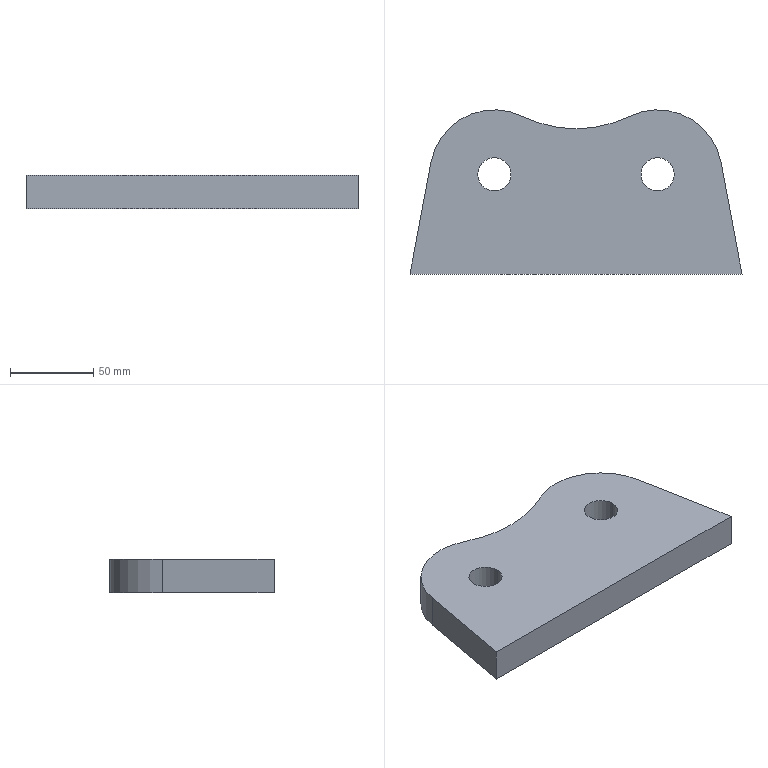Part | SolidWorks | features BaseBody 1 | 1 solid | 12 faces | box 200 x 98.946 x 20 mm | volume 325794 mm3 | cylinder 7 | plane 5 | commonest cylinder face diameters 20 x4 77.784 x2 145 x1
STEP:
#1=CARTESIAN_POINT('',(2641.622,1907.745,0.));
#2=VERTEX_POINT('',#1);
#3=CARTESIAN_POINT('',(2661.622,1907.745,0.));
#4=VERTEX_POINT('',#3);
#5=CARTESIAN_POINT('',(2651.622,1907.745,0.));
#6=DIRECTION('',(0.,0.,1.));
#7=DIRECTION('',(-1.,0.,0.));
#8=AXIS2_PLACEMENT_3D('',#5,#6,#7);
#9=CIRCLE('',#8,10.);
#10=EDGE_CURVE('',#2,#4,#9,.T.);
#11=ORIENTED_EDGE('',*,*,#10,.F.);
#12=CARTESIAN_POINT('',(2641.622,1907.745,20.));
#13=VERTEX_POINT('',#12);
#14=CARTESIAN_POINT('',(2641.622,1907.745,0.));
#15=DIRECTION('',(0.,0.,1.));
#16=VECTOR('',#15,1000.);
#17=LINE('',#14,#16);
#18=EDGE_CURVE('',#2,#13,#17,.T.);
#19=ORIENTED_EDGE('',*,*,#18,.T.);
#20=CARTESIAN_POINT('',(2661.622,1907.745,20.));
#21=VERTEX_POINT('',#20);
#22=CARTESIAN_POINT('',(2651.622,1907.745,20.));
#23=DIRECTION('',(0.,0.,1.));
#24=DIRECTION('',(-1.,0.,0.));
#25=AXIS2_PLACEMENT_3D('',#22,#23,#24);
#26=CIRCLE('',#25,10.);
#27=EDGE_CURVE('',#13,#21,#26,.T.);
#28=ORIENTED_EDGE('',*,*,#27,.T.);
#29=CARTESIAN_POINT('',(2661.622,1907.745,0.));
#30=DIRECTION('',(0.,0.,1.));
#31=VECTOR('',#30,1000.);
#32=LINE('',#29,#31);
#33=EDGE_CURVE('',#4,#21,#32,.T.);
#34=ORIENTED_EDGE('',*,*,#33,.F.);
#35=EDGE_LOOP('',(#11,#19,#28,#34));
#36=FACE_OUTER_BOUND('',#35,.T.);
#37=CARTESIAN_POINT('',(2651.622,1907.745,0.));
#38=DIRECTION('',(0.,0.,1.));
#39=DIRECTION('',(1.,0.,0.));
#40=AXIS2_PLACEMENT_3D('',#37,#38,#39);
#41=CYLINDRICAL_SURFACE('',#40,10.);
#42=ADVANCED_FACE('',(#36),#41,.F.);
#43=CARTESIAN_POINT('',(2543.258,1907.745,0.));
#44=VERTEX_POINT('',#43);
#45=CARTESIAN_POINT('',(2563.258,1907.745,0.));
#46=VERTEX_POINT('',#45);
#47=CARTESIAN_POINT('',(2553.258,1907.745,0.));
#48=DIRECTION('',(0.,0.,1.));
#49=DIRECTION('',(-1.,0.,0.));
#50=AXIS2_PLACEMENT_3D('',#47,#48,#49);
#51=CIRCLE('',#50,10.);
#52=EDGE_CURVE('',#44,#46,#51,.T.);
#53=ORIENTED_EDGE('',*,*,#52,.F.);
#54=CARTESIAN_POINT('',(2543.258,1907.745,20.));
#55=VERTEX_POINT('',#54);
#56=CARTESIAN_POINT('',(2543.258,1907.745,0.));
#57=DIRECTION('',(0.,0.,1.));
#58=VECTOR('',#57,1000.);
#59=LINE('',#56,#58);
#60=EDGE_CURVE('',#44,#55,#59,.T.);
#61=ORIENTED_EDGE('',*,*,#60,.T.);
#62=CARTESIAN_POINT('',(2563.258,1907.745,20.));
#63=VERTEX_POINT('',#62);
#64=CARTESIAN_POINT('',(2553.258,1907.745,20.));
#65=DIRECTION('',(0.,0.,1.));
#66=DIRECTION('',(-1.,0.,0.));
#67=AXIS2_PLACEMENT_3D('',#64,#65,#66);
#68=CIRCLE('',#67,10.);
#69=EDGE_CURVE('',#55,#63,#68,.T.);
#70=ORIENTED_EDGE('',*,*,#69,.T.);
#71=CARTESIAN_POINT('',(2563.258,1907.745,0.));
#72=DIRECTION('',(0.,0.,1.));
#73=VECTOR('',#72,1000.);
#74=LINE('',#71,#73);
#75=EDGE_CURVE('',#46,#63,#74,.T.);
#76=ORIENTED_EDGE('',*,*,#75,.F.);
#77=EDGE_LOOP('',(#53,#61,#70,#76));
#78=FACE_OUTER_BOUND('',#77,.T.);
#79=CARTESIAN_POINT('',(2553.258,1907.745,0.));
#80=DIRECTION('',(0.,0.,1.));
#81=DIRECTION('',(1.,0.,0.));
#82=AXIS2_PLACEMENT_3D('',#79,#80,#81);
#83=CYLINDRICAL_SURFACE('',#82,10.);
#84=ADVANCED_FACE('',(#78),#83,.F.);
#85=CARTESIAN_POINT('',(2634.451,1942.641,20.));
#86=VERTEX_POINT('',#85);
#87=CARTESIAN_POINT('',(2570.43,1942.641,20.));
#88=VERTEX_POINT('',#87);
#89=CARTESIAN_POINT('',(2602.44,2007.691,20.));
#90=DIRECTION('',(0.,0.,-1.));
#91=DIRECTION('',(-1.,0.,0.));
#92=AXIS2_PLACEMENT_3D('',#89,#90,#91);
#93=CIRCLE('',#92,72.5);
#94=EDGE_CURVE('',#86,#88,#93,.T.);
#95=ORIENTED_EDGE('',*,*,#94,.F.);
#96=CARTESIAN_POINT('',(2634.451,1942.641,0.));
#97=VERTEX_POINT('',#96);
#98=CARTESIAN_POINT('',(2634.451,1942.641,0.));
#99=DIRECTION('',(0.,0.,1.));
#100=VECTOR('',#99,1000.);
#101=LINE('',#98,#100);
#102=EDGE_CURVE('',#97,#86,#101,.T.);
#103=ORIENTED_EDGE('',*,*,#102,.F.);
#104=CARTESIAN_POINT('',(2570.43,1942.641,0.));
#105=VERTEX_POINT('',#104);
#106=CARTESIAN_POINT('',(2602.44,2007.691,0.));
#107=DIRECTION('',(0.,0.,-1.));
#108=DIRECTION('',(-1.,0.,0.));
#109=AXIS2_PLACEMENT_3D('',#106,#107,#108);
#110=CIRCLE('',#109,72.5);
#111=EDGE_CURVE('',#97,#105,#110,.T.);
#112=ORIENTED_EDGE('',*,*,#111,.T.);
#113=CARTESIAN_POINT('',(2570.43,1942.641,0.));
#114=DIRECTION('',(0.,0.,1.));
#115=VECTOR('',#114,1000.);
#116=LINE('',#113,#115);
#117=EDGE_CURVE('',#105,#88,#116,.T.);
#118=ORIENTED_EDGE('',*,*,#117,.T.);
#119=EDGE_LOOP('',(#95,#103,#112,#118));
#120=FACE_OUTER_BOUND('',#119,.T.);
#121=CARTESIAN_POINT('',(2602.44,2007.691,0.));
#122=DIRECTION('',(0.,0.,1.));
#123=DIRECTION('',(1.,0.,0.));
#124=AXIS2_PLACEMENT_3D('',#121,#122,#123);
#125=CYLINDRICAL_SURFACE('',#124,72.5);
#126=ADVANCED_FACE('',(#120),#125,.F.);
#127=CARTESIAN_POINT('',(2689.85,1914.905,20.));
#128=VERTEX_POINT('',#127);
#129=CARTESIAN_POINT('',(2651.622,1907.745,20.));
#130=DIRECTION('',(0.,0.,1.));
#131=DIRECTION('',(1.,0.,0.));
#132=AXIS2_PLACEMENT_3D('',#129,#130,#131);
#133=CIRCLE('',#132,38.892);
#134=EDGE_CURVE('',#128,#86,#133,.T.);
#135=ORIENTED_EDGE('',*,*,#134,.F.);
#136=CARTESIAN_POINT('',(2689.85,1914.905,0.));
#137=VERTEX_POINT('',#136);
#138=CARTESIAN_POINT('',(2689.85,1914.905,0.));
#139=DIRECTION('',(0.,0.,1.));
#140=VECTOR('',#139,1000.);
#141=LINE('',#138,#140);
#142=EDGE_CURVE('',#137,#128,#141,.T.);
#143=ORIENTED_EDGE('',*,*,#142,.F.);
#144=CARTESIAN_POINT('',(2651.622,1907.745,0.));
#145=DIRECTION('',(0.,0.,1.));
#146=DIRECTION('',(1.,0.,0.));
#147=AXIS2_PLACEMENT_3D('',#144,#145,#146);
#148=CIRCLE('',#147,38.892);
#149=EDGE_CURVE('',#137,#97,#148,.T.);
#150=ORIENTED_EDGE('',*,*,#149,.T.);
#151=ORIENTED_EDGE('',*,*,#102,.T.);
#152=EDGE_LOOP('',(#135,#143,#150,#151));
#153=FACE_OUTER_BOUND('',#152,.T.);
#154=CARTESIAN_POINT('',(2651.622,1907.745,0.));
#155=DIRECTION('',(0.,0.,1.));
#156=DIRECTION('',(1.,0.,0.));
#157=AXIS2_PLACEMENT_3D('',#154,#155,#156);
#158=CYLINDRICAL_SURFACE('',#157,38.892);
#159=ADVANCED_FACE('',(#153),#158,.T.);
#160=CARTESIAN_POINT('',(2702.44,1847.691,20.));
#161=VERTEX_POINT('',#160);
#162=CARTESIAN_POINT('',(2702.44,1847.691,20.));
#163=DIRECTION('',(-0.1841,0.9829,0.));
#164=VECTOR('',#163,1000.);
#165=LINE('',#162,#164);
#166=EDGE_CURVE('',#161,#128,#165,.T.);
#167=ORIENTED_EDGE('',*,*,#166,.F.);
#168=CARTESIAN_POINT('',(2702.44,1847.691,0.));
#169=VERTEX_POINT('',#168);
#170=CARTESIAN_POINT('',(2702.44,1847.691,0.));
#171=DIRECTION('',(0.,0.,1.));
#172=VECTOR('',#171,1000.);
#173=LINE('',#170,#172);
#174=EDGE_CURVE('',#169,#161,#173,.T.);
#175=ORIENTED_EDGE('',*,*,#174,.F.);
#176=CARTESIAN_POINT('',(2702.44,1847.691,0.));
#177=DIRECTION('',(-0.1841,0.9829,0.));
#178=VECTOR('',#177,1000.);
#179=LINE('',#176,#178);
#180=EDGE_CURVE('',#169,#137,#179,.T.);
#181=ORIENTED_EDGE('',*,*,#180,.T.);
#182=ORIENTED_EDGE('',*,*,#142,.T.);
#183=EDGE_LOOP('',(#167,#175,#181,#182));
#184=FACE_OUTER_BOUND('',#183,.T.);
#185=CARTESIAN_POINT('',(2702.44,1847.691,0.));
#186=DIRECTION('',(0.9829,0.1841,0.));
#187=DIRECTION('',(-0.1841,0.9829,0.));
#188=AXIS2_PLACEMENT_3D('',#185,#186,#187);
#189=PLANE('',#188);
#190=ADVANCED_FACE('',(#184),#189,.T.);
#191=CARTESIAN_POINT('',(2502.44,1847.691,20.));
#192=VERTEX_POINT('',#191);
#193=CARTESIAN_POINT('',(2502.44,1847.691,20.));
#194=DIRECTION('',(1.,0.,0.));
#195=VECTOR('',#194,1000.);
#196=LINE('',#193,#195);
#197=EDGE_CURVE('',#192,#161,#196,.T.);
#198=ORIENTED_EDGE('',*,*,#197,.F.);
#199=CARTESIAN_POINT('',(2502.44,1847.691,0.));
#200=VERTEX_POINT('',#199);
#201=CARTESIAN_POINT('',(2502.44,1847.691,0.));
#202=DIRECTION('',(0.,0.,1.));
#203=VECTOR('',#202,1000.);
#204=LINE('',#201,#203);
#205=EDGE_CURVE('',#200,#192,#204,.T.);
#206=ORIENTED_EDGE('',*,*,#205,.F.);
#207=CARTESIAN_POINT('',(2502.44,1847.691,0.));
#208=DIRECTION('',(1.,0.,0.));
#209=VECTOR('',#208,1000.);
#210=LINE('',#207,#209);
#211=EDGE_CURVE('',#200,#169,#210,.T.);
#212=ORIENTED_EDGE('',*,*,#211,.T.);
#213=ORIENTED_EDGE('',*,*,#174,.T.);
#214=EDGE_LOOP('',(#198,#206,#212,#213));
#215=FACE_OUTER_BOUND('',#214,.T.);
#216=CARTESIAN_POINT('',(2502.44,1847.691,0.));
#217=DIRECTION('',(0.,-1.,0.));
#218=DIRECTION('',(0.,0.,-1.));
#219=AXIS2_PLACEMENT_3D('',#216,#217,#218);
#220=PLANE('',#219);
#221=ADVANCED_FACE('',(#215),#220,.T.);
#222=CARTESIAN_POINT('',(2515.031,1914.905,20.));
#223=VERTEX_POINT('',#222);
#224=CARTESIAN_POINT('',(2515.031,1914.905,20.));
#225=DIRECTION('',(-0.1841,-0.9829,0.));
#226=VECTOR('',#225,1000.);
#227=LINE('',#224,#226);
#228=EDGE_CURVE('',#223,#192,#227,.T.);
#229=ORIENTED_EDGE('',*,*,#228,.F.);
#230=CARTESIAN_POINT('',(2515.031,1914.905,0.));
#231=VERTEX_POINT('',#230);
#232=CARTESIAN_POINT('',(2515.031,1914.905,0.));
#233=DIRECTION('',(0.,0.,1.));
#234=VECTOR('',#233,1000.);
#235=LINE('',#232,#234);
#236=EDGE_CURVE('',#231,#223,#235,.T.);
#237=ORIENTED_EDGE('',*,*,#236,.F.);
#238=CARTESIAN_POINT('',(2515.031,1914.905,0.));
#239=DIRECTION('',(-0.1841,-0.9829,0.));
#240=VECTOR('',#239,1000.);
#241=LINE('',#238,#240);
#242=EDGE_CURVE('',#231,#200,#241,.T.);
#243=ORIENTED_EDGE('',*,*,#242,.T.);
#244=ORIENTED_EDGE('',*,*,#205,.T.);
#245=EDGE_LOOP('',(#229,#237,#243,#244));
#246=FACE_OUTER_BOUND('',#245,.T.);
#247=CARTESIAN_POINT('',(2515.031,1914.905,0.));
#248=DIRECTION('',(-0.9829,0.1841,0.));
#249=DIRECTION('',(-0.1841,-0.9829,0.));
#250=AXIS2_PLACEMENT_3D('',#247,#248,#249);
#251=PLANE('',#250);
#252=ADVANCED_FACE('',(#246),#251,.T.);
#253=CARTESIAN_POINT('',(2553.258,1907.745,20.));
#254=DIRECTION('',(0.,0.,1.));
#255=DIRECTION('',(1.,0.,0.));
#256=AXIS2_PLACEMENT_3D('',#253,#254,#255);
#257=CIRCLE('',#256,38.892);
#258=EDGE_CURVE('',#88,#223,#257,.T.);
#259=ORIENTED_EDGE('',*,*,#258,.F.);
#260=ORIENTED_EDGE('',*,*,#117,.F.);
#261=CARTESIAN_POINT('',(2553.258,1907.745,0.));
#262=DIRECTION('',(0.,0.,1.));
#263=DIRECTION('',(1.,0.,0.));
#264=AXIS2_PLACEMENT_3D('',#261,#262,#263);
#265=CIRCLE('',#264,38.892);
#266=EDGE_CURVE('',#105,#231,#265,.T.);
#267=ORIENTED_EDGE('',*,*,#266,.T.);
#268=ORIENTED_EDGE('',*,*,#236,.T.);
#269=EDGE_LOOP('',(#259,#260,#267,#268));
#270=FACE_OUTER_BOUND('',#269,.T.);
#271=CARTESIAN_POINT('',(2553.258,1907.745,0.));
#272=DIRECTION('',(0.,0.,1.));
#273=DIRECTION('',(1.,0.,0.));
#274=AXIS2_PLACEMENT_3D('',#271,#272,#273);
#275=CYLINDRICAL_SURFACE('',#274,38.892);
#276=ADVANCED_FACE('',(#270),#275,.T.);
#277=CARTESIAN_POINT('',(2651.622,1907.745,0.));
#278=DIRECTION('',(0.,0.,1.));
#279=DIRECTION('',(-1.,0.,0.));
#280=AXIS2_PLACEMENT_3D('',#277,#278,#279);
#281=CIRCLE('',#280,10.);
#282=EDGE_CURVE('',#4,#2,#281,.T.);
#283=ORIENTED_EDGE('',*,*,#282,.T.);
#284=ORIENTED_EDGE('',*,*,#10,.T.);
#285=EDGE_LOOP('',(#283,#284));
#286=FACE_BOUND('',#285,.T.);
#287=CARTESIAN_POINT('',(2553.258,1907.745,0.));
#288=DIRECTION('',(0.,0.,1.));
#289=DIRECTION('',(-1.,0.,0.));
#290=AXIS2_PLACEMENT_3D('',#287,#288,#289);
#291=CIRCLE('',#290,10.);
#292=EDGE_CURVE('',#46,#44,#291,.T.);
#293=ORIENTED_EDGE('',*,*,#292,.T.);
#294=ORIENTED_EDGE('',*,*,#52,.T.);
#295=EDGE_LOOP('',(#293,#294));
#296=FACE_BOUND('',#295,.T.);
#297=ORIENTED_EDGE('',*,*,#111,.F.);
#298=ORIENTED_EDGE('',*,*,#149,.F.);
#299=ORIENTED_EDGE('',*,*,#180,.F.);
#300=ORIENTED_EDGE('',*,*,#211,.F.);
#301=ORIENTED_EDGE('',*,*,#242,.F.);
#302=ORIENTED_EDGE('',*,*,#266,.F.);
#303=EDGE_LOOP('',(#297,#298,#299,#300,#301,#302));
#304=FACE_OUTER_BOUND('',#303,.T.);
#305=CARTESIAN_POINT('',(2602.44,2007.691,0.));
#306=DIRECTION('',(0.,0.,-1.));
#307=DIRECTION('',(-1.,0.,0.));
#308=AXIS2_PLACEMENT_3D('',#305,#306,#307);
#309=PLANE('',#308);
#310=ADVANCED_FACE('',(#286,#296,#304),#309,.T.);
#311=CARTESIAN_POINT('',(2651.622,1907.745,20.));
#312=DIRECTION('',(0.,0.,1.));
#313=DIRECTION('',(-1.,0.,0.));
#314=AXIS2_PLACEMENT_3D('',#311,#312,#313);
#315=CIRCLE('',#314,10.);
#316=EDGE_CURVE('',#21,#13,#315,.T.);
#317=ORIENTED_EDGE('',*,*,#316,.F.);
#318=ORIENTED_EDGE('',*,*,#27,.F.);
#319=EDGE_LOOP('',(#317,#318));
#320=FACE_BOUND('',#319,.T.);
#321=CARTESIAN_POINT('',(2553.258,1907.745,20.));
#322=DIRECTION('',(0.,0.,1.));
#323=DIRECTION('',(-1.,0.,0.));
#324=AXIS2_PLACEMENT_3D('',#321,#322,#323);
#325=CIRCLE('',#324,10.);
#326=EDGE_CURVE('',#63,#55,#325,.T.);
#327=ORIENTED_EDGE('',*,*,#326,.F.);
#328=ORIENTED_EDGE('',*,*,#69,.F.);
#329=EDGE_LOOP('',(#327,#328));
#330=FACE_BOUND('',#329,.T.);
#331=ORIENTED_EDGE('',*,*,#94,.T.);
#332=ORIENTED_EDGE('',*,*,#258,.T.);
#333=ORIENTED_EDGE('',*,*,#228,.T.);
#334=ORIENTED_EDGE('',*,*,#197,.T.);
#335=ORIENTED_EDGE('',*,*,#166,.T.);
#336=ORIENTED_EDGE('',*,*,#134,.T.);
#337=EDGE_LOOP('',(#331,#332,#333,#334,#335,#336));
#338=FACE_OUTER_BOUND('',#337,.T.);
#339=CARTESIAN_POINT('',(2602.44,2007.691,20.));
#340=DIRECTION('',(0.,0.,-1.));
#341=DIRECTION('',(-1.,0.,0.));
#342=AXIS2_PLACEMENT_3D('',#339,#340,#341);
#343=PLANE('',#342);
#344=ADVANCED_FACE('',(#320,#330,#338),#343,.F.);
#345=ORIENTED_EDGE('',*,*,#60,.F.);
#346=ORIENTED_EDGE('',*,*,#292,.F.);
#347=ORIENTED_EDGE('',*,*,#75,.T.);
#348=ORIENTED_EDGE('',*,*,#326,.T.);
#349=EDGE_LOOP('',(#345,#346,#347,#348));
#350=FACE_OUTER_BOUND('',#349,.T.);
#351=CARTESIAN_POINT('',(2553.258,1907.745,0.));
#352=DIRECTION('',(0.,0.,1.));
#353=DIRECTION('',(1.,0.,0.));
#354=AXIS2_PLACEMENT_3D('',#351,#352,#353);
#355=CYLINDRICAL_SURFACE('',#354,10.);
#356=ADVANCED_FACE('',(#350),#355,.F.);
#357=ORIENTED_EDGE('',*,*,#18,.F.);
#358=ORIENTED_EDGE('',*,*,#282,.F.);
#359=ORIENTED_EDGE('',*,*,#33,.T.);
#360=ORIENTED_EDGE('',*,*,#316,.T.);
#361=EDGE_LOOP('',(#357,#358,#359,#360));
#362=FACE_OUTER_BOUND('',#361,.T.);
#363=CARTESIAN_POINT('',(2651.622,1907.745,0.));
#364=DIRECTION('',(0.,0.,1.));
#365=DIRECTION('',(1.,0.,0.));
#366=AXIS2_PLACEMENT_3D('',#363,#364,#365);
#367=CYLINDRICAL_SURFACE('',#366,10.);
#368=ADVANCED_FACE('',(#362),#367,.F.);
#369=CLOSED_SHELL('',(#42,#84,#126,#159,#190,#221,#252,#276,#310,#344,#356,#368));
#370=MANIFOLD_SOLID_BREP('',#369);
#371=CARTESIAN_POINT('',(0.,0.,0.));
#372=DIRECTION('',(0.,0.,1.));
#373=DIRECTION('',(1.,0.,0.));
#374=AXIS2_PLACEMENT_3D('',#371,#372,#373);
#375=(LENGTH_UNIT()NAMED_UNIT(*)SI_UNIT(.MILLI.,.METRE.));
#376=UNCERTAINTY_MEASURE_WITH_UNIT(LENGTH_MEASURE(0.00001),#375,'','');
#377=(NAMED_UNIT(*)PLANE_ANGLE_UNIT()SI_UNIT($,.RADIAN.));
#378=(NAMED_UNIT(*)SI_UNIT($,.STERADIAN.)SOLID_ANGLE_UNIT());
#379=(GEOMETRIC_REPRESENTATION_CONTEXT(3)GLOBAL_UNCERTAINTY_ASSIGNED_CONTEXT((#376))GLOBAL_UNIT_ASSIGNED_CONTEXT((#375,#377,#378))REPRESENTATION_CONTEXT('',''));
#380=ADVANCED_BREP_SHAPE_REPRESENTATION('',(#370,#374),#379);